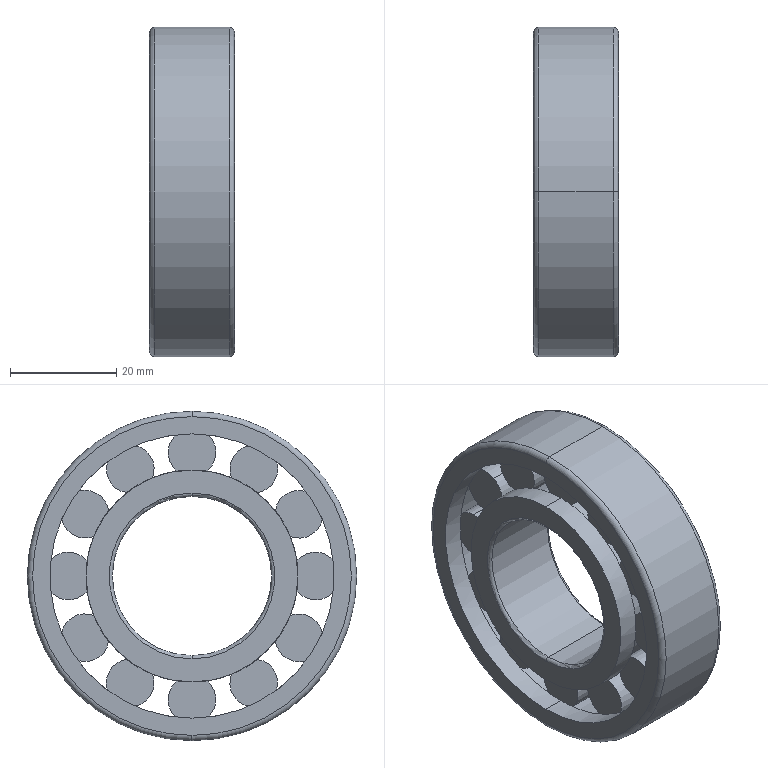Part | SolidWorks | features Revolution 3, CirPattern 1 | 1 solid | 156 faces | box 16 x 62 x 62 mm | volume 24506 mm3 | plane 76 | cylinder 72 | torus 8 | commonest cylinder face diameters 9 x36 37.5 x12 55.5 x12 39.9 x4 53.5 x4 30 x2